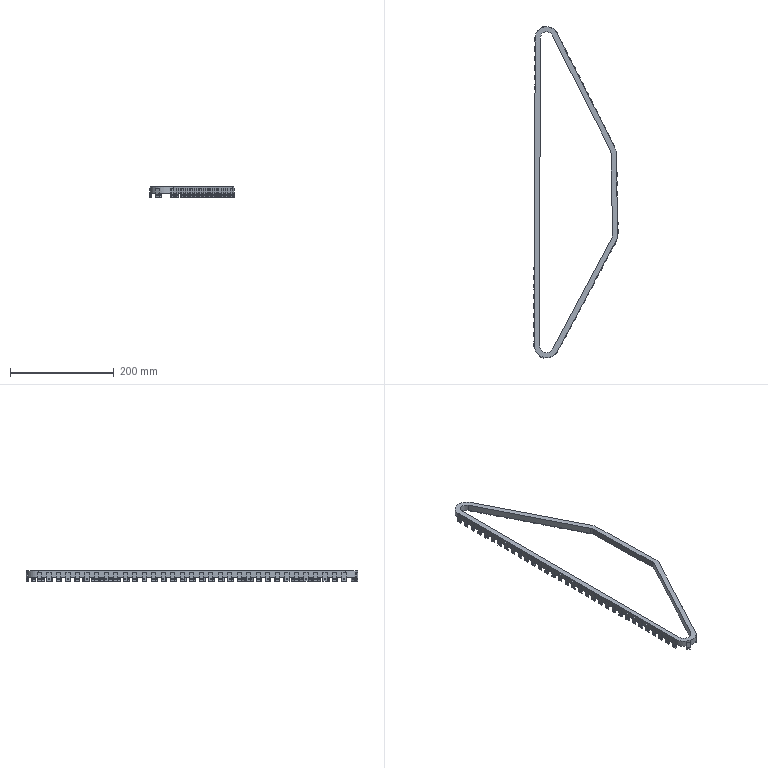Part | STEP file | Belt 1 | 1 solid | 596 faces | box 163.112 x 641.3 x 20 mm | volume 175468 mm3 | plane 442 | cylinder 154 | commonest cylinder face diameters 3 x144 24 x2 27.295 x2 44 x2 47.295 x2 30 x1